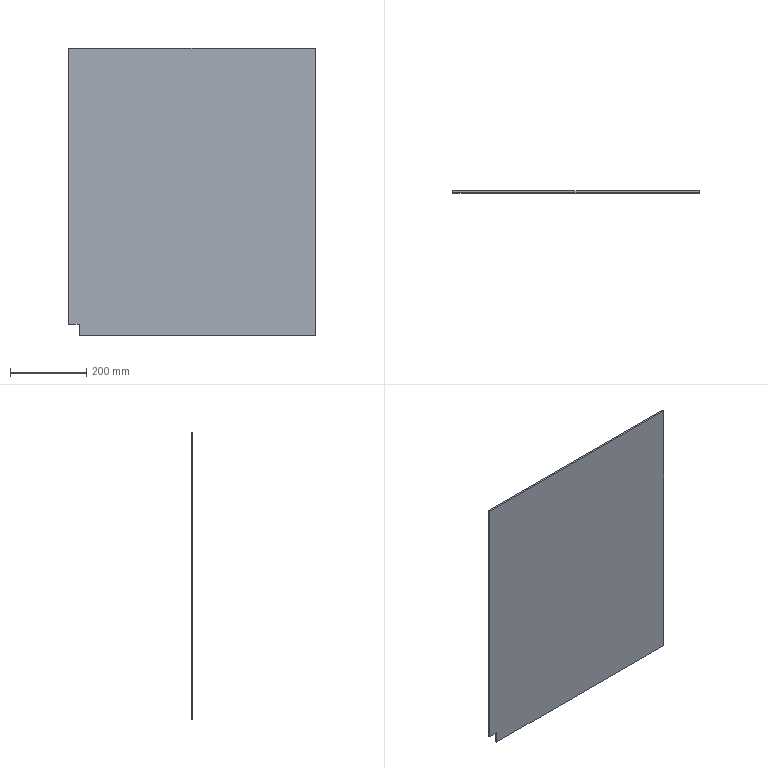Part | SolidWorks | features BaseBody 1, ICE 1 | 1 solid | 8 faces | box 647 x 5 x 755 mm | volume 2438375 mm3 | plane 8
STEP:
#1=CARTESIAN_POINT('',(87.,40.,360.));
#2=VERTEX_POINT('',#1);
#3=CARTESIAN_POINT('',(87.,40.,-395.));
#4=VERTEX_POINT('',#3);
#5=CARTESIAN_POINT('',(87.,40.,-17.5));
#6=DIRECTION('',(0.,0.,-1.));
#7=VECTOR('',#6,1000.);
#8=LINE('',#5,#7);
#9=EDGE_CURVE('',#2,#4,#8,.T.);
#10=ORIENTED_EDGE('',*,*,#9,.F.);
#11=CARTESIAN_POINT('',(-560.,40.,360.));
#12=VERTEX_POINT('',#11);
#13=CARTESIAN_POINT('',(-560.,40.,360.));
#14=DIRECTION('',(1.,0.,0.));
#15=VECTOR('',#14,1000.);
#16=LINE('',#13,#15);
#17=EDGE_CURVE('',#12,#2,#16,.T.);
#18=ORIENTED_EDGE('',*,*,#17,.F.);
#19=CARTESIAN_POINT('',(-560.,40.,-365.));
#20=VERTEX_POINT('',#19);
#21=CARTESIAN_POINT('',(-560.,40.,-365.));
#22=DIRECTION('',(0.,0.,1.));
#23=VECTOR('',#22,1000.);
#24=LINE('',#21,#23);
#25=EDGE_CURVE('',#20,#12,#24,.T.);
#26=ORIENTED_EDGE('',*,*,#25,.F.);
#27=CARTESIAN_POINT('',(-533.,40.,-365.));
#28=VERTEX_POINT('',#27);
#29=CARTESIAN_POINT('',(-533.,40.,-365.));
#30=DIRECTION('',(-1.,0.,0.));
#31=VECTOR('',#30,1000.);
#32=LINE('',#29,#31);
#33=EDGE_CURVE('',#28,#20,#32,.T.);
#34=ORIENTED_EDGE('',*,*,#33,.F.);
#35=CARTESIAN_POINT('',(-533.,40.,-395.));
#36=VERTEX_POINT('',#35);
#37=CARTESIAN_POINT('',(-533.,40.,-395.));
#38=DIRECTION('',(0.,0.,1.));
#39=VECTOR('',#38,1000.);
#40=LINE('',#37,#39);
#41=EDGE_CURVE('',#36,#28,#40,.T.);
#42=ORIENTED_EDGE('',*,*,#41,.F.);
#43=CARTESIAN_POINT('',(533.,40.,-395.));
#44=DIRECTION('',(-1.,0.,0.));
#45=VECTOR('',#44,1000.);
#46=LINE('',#43,#45);
#47=EDGE_CURVE('',#4,#36,#46,.T.);
#48=ORIENTED_EDGE('',*,*,#47,.F.);
#49=EDGE_LOOP('',(#10,#18,#26,#34,#42,#48));
#50=FACE_OUTER_BOUND('',#49,.T.);
#51=CARTESIAN_POINT('',(0.,40.,-17.5));
#52=DIRECTION('',(0.,-1.,0.));
#53=DIRECTION('',(0.,0.,-1.));
#54=AXIS2_PLACEMENT_3D('',#51,#52,#53);
#55=PLANE('',#54);
#56=ADVANCED_FACE('',(#50),#55,.T.);
#57=CARTESIAN_POINT('',(87.,45.,-395.));
#58=VERTEX_POINT('',#57);
#59=CARTESIAN_POINT('',(87.,45.,360.));
#60=VERTEX_POINT('',#59);
#61=CARTESIAN_POINT('',(87.,45.,360.));
#62=DIRECTION('',(0.,0.,1.));
#63=VECTOR('',#62,1000.);
#64=LINE('',#61,#63);
#65=EDGE_CURVE('',#58,#60,#64,.T.);
#66=ORIENTED_EDGE('',*,*,#65,.F.);
#67=CARTESIAN_POINT('',(-533.,45.,-395.));
#68=VERTEX_POINT('',#67);
#69=CARTESIAN_POINT('',(-533.,45.,-395.));
#70=DIRECTION('',(1.,0.,0.));
#71=VECTOR('',#70,1000.);
#72=LINE('',#69,#71);
#73=EDGE_CURVE('',#68,#58,#72,.T.);
#74=ORIENTED_EDGE('',*,*,#73,.F.);
#75=CARTESIAN_POINT('',(-533.,45.,-365.));
#76=VERTEX_POINT('',#75);
#77=CARTESIAN_POINT('',(-533.,45.,-365.));
#78=DIRECTION('',(0.,0.,-1.));
#79=VECTOR('',#78,1000.);
#80=LINE('',#77,#79);
#81=EDGE_CURVE('',#76,#68,#80,.T.);
#82=ORIENTED_EDGE('',*,*,#81,.F.);
#83=CARTESIAN_POINT('',(-560.,45.,-365.));
#84=VERTEX_POINT('',#83);
#85=CARTESIAN_POINT('',(-560.,45.,-365.));
#86=DIRECTION('',(1.,0.,0.));
#87=VECTOR('',#86,1000.);
#88=LINE('',#85,#87);
#89=EDGE_CURVE('',#84,#76,#88,.T.);
#90=ORIENTED_EDGE('',*,*,#89,.F.);
#91=CARTESIAN_POINT('',(-560.,45.,360.));
#92=VERTEX_POINT('',#91);
#93=CARTESIAN_POINT('',(-560.,45.,360.));
#94=DIRECTION('',(0.,0.,-1.));
#95=VECTOR('',#94,1000.);
#96=LINE('',#93,#95);
#97=EDGE_CURVE('',#92,#84,#96,.T.);
#98=ORIENTED_EDGE('',*,*,#97,.F.);
#99=CARTESIAN_POINT('',(560.,45.,360.));
#100=DIRECTION('',(-1.,0.,0.));
#101=VECTOR('',#100,1000.);
#102=LINE('',#99,#101);
#103=EDGE_CURVE('',#60,#92,#102,.T.);
#104=ORIENTED_EDGE('',*,*,#103,.F.);
#105=EDGE_LOOP('',(#66,#74,#82,#90,#98,#104));
#106=FACE_OUTER_BOUND('',#105,.T.);
#107=CARTESIAN_POINT('',(0.,45.,-17.5));
#108=DIRECTION('',(0.,1.,0.));
#109=DIRECTION('',(1.,0.,0.));
#110=AXIS2_PLACEMENT_3D('',#107,#108,#109);
#111=PLANE('',#110);
#112=ADVANCED_FACE('',(#106),#111,.T.);
#113=ORIENTED_EDGE('',*,*,#33,.T.);
#114=CARTESIAN_POINT('',(-560.,45.,-365.));
#115=DIRECTION('',(0.,-1.,0.));
#116=VECTOR('',#115,1000.);
#117=LINE('',#114,#116);
#118=EDGE_CURVE('',#84,#20,#117,.T.);
#119=ORIENTED_EDGE('',*,*,#118,.F.);
#120=ORIENTED_EDGE('',*,*,#89,.T.);
#121=CARTESIAN_POINT('',(-533.,40.,-365.));
#122=DIRECTION('',(0.,1.,0.));
#123=VECTOR('',#122,1000.);
#124=LINE('',#121,#123);
#125=EDGE_CURVE('',#28,#76,#124,.T.);
#126=ORIENTED_EDGE('',*,*,#125,.F.);
#127=EDGE_LOOP('',(#113,#119,#120,#126));
#128=FACE_OUTER_BOUND('',#127,.T.);
#129=CARTESIAN_POINT('',(-533.,40.,-365.));
#130=DIRECTION('',(0.,0.,-1.));
#131=DIRECTION('',(0.,-1.,0.));
#132=AXIS2_PLACEMENT_3D('',#129,#130,#131);
#133=PLANE('',#132);
#134=ADVANCED_FACE('',(#128),#133,.T.);
#135=ORIENTED_EDGE('',*,*,#25,.T.);
#136=CARTESIAN_POINT('',(-560.,45.,360.));
#137=DIRECTION('',(0.,-1.,0.));
#138=VECTOR('',#137,1000.);
#139=LINE('',#136,#138);
#140=EDGE_CURVE('',#92,#12,#139,.T.);
#141=ORIENTED_EDGE('',*,*,#140,.F.);
#142=ORIENTED_EDGE('',*,*,#97,.T.);
#143=ORIENTED_EDGE('',*,*,#118,.T.);
#144=EDGE_LOOP('',(#135,#141,#142,#143));
#145=FACE_OUTER_BOUND('',#144,.T.);
#146=CARTESIAN_POINT('',(-560.,40.,-365.));
#147=DIRECTION('',(-1.,0.,0.));
#148=DIRECTION('',(0.,0.,1.));
#149=AXIS2_PLACEMENT_3D('',#146,#147,#148);
#150=PLANE('',#149);
#151=ADVANCED_FACE('',(#145),#150,.T.);
#152=CARTESIAN_POINT('',(87.,35.,360.));
#153=DIRECTION('',(0.,1.,0.));
#154=VECTOR('',#153,1000.);
#155=LINE('',#152,#154);
#156=EDGE_CURVE('',#2,#60,#155,.T.);
#157=ORIENTED_EDGE('',*,*,#156,.T.);
#158=ORIENTED_EDGE('',*,*,#103,.T.);
#159=ORIENTED_EDGE('',*,*,#140,.T.);
#160=ORIENTED_EDGE('',*,*,#17,.T.);
#161=EDGE_LOOP('',(#157,#158,#159,#160));
#162=FACE_OUTER_BOUND('',#161,.T.);
#163=CARTESIAN_POINT('',(-560.,40.,360.));
#164=DIRECTION('',(0.,0.,1.));
#165=DIRECTION('',(1.,0.,0.));
#166=AXIS2_PLACEMENT_3D('',#163,#164,#165);
#167=PLANE('',#166);
#168=ADVANCED_FACE('',(#162),#167,.T.);
#169=CARTESIAN_POINT('',(87.,40.,-395.));
#170=DIRECTION('',(0.,1.,0.));
#171=VECTOR('',#170,1000.);
#172=LINE('',#169,#171);
#173=EDGE_CURVE('',#4,#58,#172,.T.);
#174=ORIENTED_EDGE('',*,*,#173,.F.);
#175=ORIENTED_EDGE('',*,*,#47,.T.);
#176=CARTESIAN_POINT('',(-533.,45.,-395.));
#177=DIRECTION('',(0.,-1.,0.));
#178=VECTOR('',#177,1000.);
#179=LINE('',#176,#178);
#180=EDGE_CURVE('',#68,#36,#179,.T.);
#181=ORIENTED_EDGE('',*,*,#180,.F.);
#182=ORIENTED_EDGE('',*,*,#73,.T.);
#183=EDGE_LOOP('',(#174,#175,#181,#182));
#184=FACE_OUTER_BOUND('',#183,.T.);
#185=CARTESIAN_POINT('',(533.,40.,-395.));
#186=DIRECTION('',(0.,0.,-1.));
#187=DIRECTION('',(0.,-1.,0.));
#188=AXIS2_PLACEMENT_3D('',#185,#186,#187);
#189=PLANE('',#188);
#190=ADVANCED_FACE('',(#184),#189,.T.);
#191=ORIENTED_EDGE('',*,*,#41,.T.);
#192=ORIENTED_EDGE('',*,*,#125,.T.);
#193=ORIENTED_EDGE('',*,*,#81,.T.);
#194=ORIENTED_EDGE('',*,*,#180,.T.);
#195=EDGE_LOOP('',(#191,#192,#193,#194));
#196=FACE_OUTER_BOUND('',#195,.T.);
#197=CARTESIAN_POINT('',(-533.,40.,-395.));
#198=DIRECTION('',(-1.,0.,0.));
#199=DIRECTION('',(0.,0.,1.));
#200=AXIS2_PLACEMENT_3D('',#197,#198,#199);
#201=PLANE('',#200);
#202=ADVANCED_FACE('',(#196),#201,.T.);
#203=ORIENTED_EDGE('',*,*,#9,.T.);
#204=ORIENTED_EDGE('',*,*,#173,.T.);
#205=ORIENTED_EDGE('',*,*,#65,.T.);
#206=ORIENTED_EDGE('',*,*,#156,.F.);
#207=EDGE_LOOP('',(#203,#204,#205,#206));
#208=FACE_OUTER_BOUND('',#207,.T.);
#209=CARTESIAN_POINT('',(87.,35.,360.));
#210=DIRECTION('',(-1.,0.,0.));
#211=DIRECTION('',(0.,0.,1.));
#212=AXIS2_PLACEMENT_3D('',#209,#210,#211);
#213=PLANE('',#212);
#214=ADVANCED_FACE('',(#208),#213,.F.);
#215=CLOSED_SHELL('',(#56,#112,#134,#151,#168,#190,#202,#214));
#216=MANIFOLD_SOLID_BREP('',#215);
#217=CARTESIAN_POINT('',(0.,0.,0.));
#218=DIRECTION('',(0.,0.,1.));
#219=DIRECTION('',(1.,0.,0.));
#220=AXIS2_PLACEMENT_3D('',#217,#218,#219);
#221=(LENGTH_UNIT()NAMED_UNIT(*)SI_UNIT(.MILLI.,.METRE.));
#222=UNCERTAINTY_MEASURE_WITH_UNIT(LENGTH_MEASURE(0.00001),#221,'','');
#223=(NAMED_UNIT(*)PLANE_ANGLE_UNIT()SI_UNIT($,.RADIAN.));
#224=(NAMED_UNIT(*)SI_UNIT($,.STERADIAN.)SOLID_ANGLE_UNIT());
#225=(GEOMETRIC_REPRESENTATION_CONTEXT(3)GLOBAL_UNCERTAINTY_ASSIGNED_CONTEXT((#222))GLOBAL_UNIT_ASSIGNED_CONTEXT((#221,#223,#224))REPRESENTATION_CONTEXT('',''));
#226=ADVANCED_BREP_SHAPE_REPRESENTATION('',(#216,#220),#225);